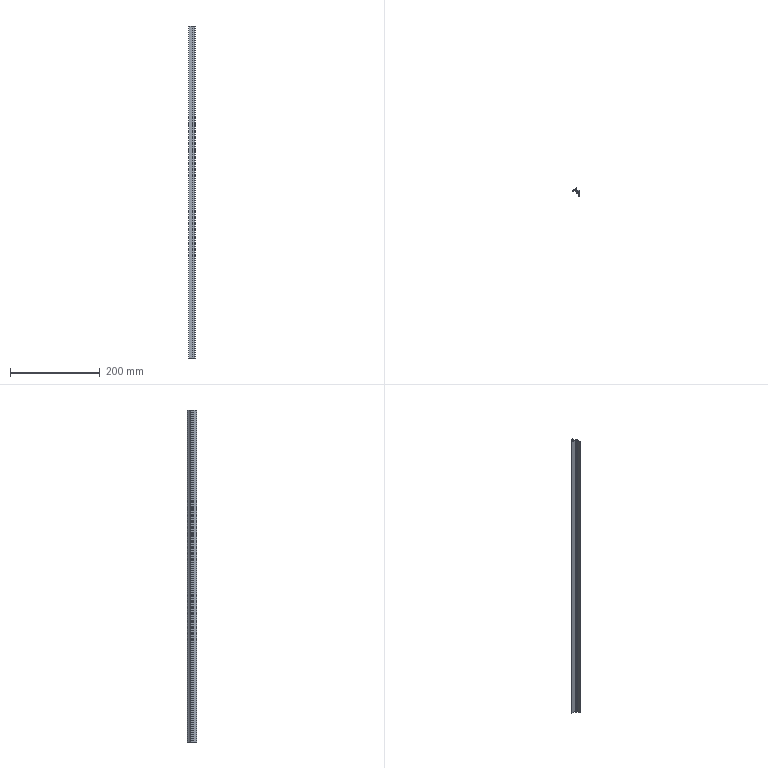Part | SolidWorks | features BaseBody 1, ICE 1, MoveFace 1 | 1 solid | 27 faces | box 14 x 20.3 x 740 mm | volume 37678 mm3 | plane 20 | cylinder 7 | commonest cylinder face diameters 0.387 x2 0.8 x2 0.4 x1 20 x1 22 x1
STEP:
#1=CARTESIAN_POINT('',(-5.304,-0.625,200.));
#2=VERTEX_POINT('',#1);
#3=CARTESIAN_POINT('',(-5.449,-0.8125,200.));
#4=VERTEX_POINT('',#3);
#5=CARTESIAN_POINT('',(-5.255,-0.8125,200.));
#6=DIRECTION('',(0.,0.,1.));
#7=DIRECTION('',(-1.,0.,0.));
#8=AXIS2_PLACEMENT_3D('',#5,#6,#7);
#9=CIRCLE('',#8,0.1937);
#10=EDGE_CURVE('',#2,#4,#9,.T.);
#11=ORIENTED_EDGE('',*,*,#10,.T.);
#12=CARTESIAN_POINT('',(-5.449,-0.8125,-540.));
#13=VERTEX_POINT('',#12);
#14=CARTESIAN_POINT('',(-5.449,-0.8125,230.));
#15=DIRECTION('',(0.,0.,-1.));
#16=VECTOR('',#15,1000.);
#17=LINE('',#14,#16);
#18=EDGE_CURVE('',#4,#13,#17,.T.);
#19=ORIENTED_EDGE('',*,*,#18,.T.);
#20=CARTESIAN_POINT('',(-5.304,-0.625,-540.));
#21=VERTEX_POINT('',#20);
#22=CARTESIAN_POINT('',(-5.255,-0.8125,-540.));
#23=DIRECTION('',(0.,0.,-1.));
#24=DIRECTION('',(1.,0.,0.));
#25=AXIS2_PLACEMENT_3D('',#22,#23,#24);
#26=CIRCLE('',#25,0.1937);
#27=EDGE_CURVE('',#13,#21,#26,.T.);
#28=ORIENTED_EDGE('',*,*,#27,.T.);
#29=CARTESIAN_POINT('',(-5.304,-0.625,230.));
#30=DIRECTION('',(0.,0.,-1.));
#31=VECTOR('',#30,1000.);
#32=LINE('',#29,#31);
#33=EDGE_CURVE('',#2,#21,#32,.T.);
#34=ORIENTED_EDGE('',*,*,#33,.F.);
#35=EDGE_LOOP('',(#11,#19,#28,#34));
#36=FACE_OUTER_BOUND('',#35,.T.);
#37=CARTESIAN_POINT('',(-5.255,-0.8125,230.));
#38=DIRECTION('',(0.,0.,-1.));
#39=DIRECTION('',(-1.,0.,0.));
#40=AXIS2_PLACEMENT_3D('',#37,#38,#39);
#41=CYLINDRICAL_SURFACE('',#40,0.1937);
#42=ADVANCED_FACE('',(#36),#41,.F.);
#43=CARTESIAN_POINT('',(5.,-1.,-540.));
#44=VERTEX_POINT('',#43);
#45=CARTESIAN_POINT('',(5.,-14.3,-540.));
#46=VERTEX_POINT('',#45);
#47=CARTESIAN_POINT('',(5.,29.623,-540.));
#48=DIRECTION('',(0.,-1.,0.));
#49=VECTOR('',#48,1000.);
#50=LINE('',#47,#49);
#51=EDGE_CURVE('',#44,#46,#50,.T.);
#52=ORIENTED_EDGE('',*,*,#51,.F.);
#53=CARTESIAN_POINT('',(5.,-1.,200.));
#54=VERTEX_POINT('',#53);
#55=CARTESIAN_POINT('',(5.,-1.,230.));
#56=DIRECTION('',(0.,0.,-1.));
#57=VECTOR('',#56,1000.);
#58=LINE('',#55,#57);
#59=EDGE_CURVE('',#54,#44,#58,.T.);
#60=ORIENTED_EDGE('',*,*,#59,.F.);
#61=CARTESIAN_POINT('',(5.,-14.3,200.));
#62=VERTEX_POINT('',#61);
#63=CARTESIAN_POINT('',(5.,-14.3,200.));
#64=DIRECTION('',(0.,1.,0.));
#65=VECTOR('',#64,1000.);
#66=LINE('',#63,#65);
#67=EDGE_CURVE('',#62,#54,#66,.T.);
#68=ORIENTED_EDGE('',*,*,#67,.F.);
#69=CARTESIAN_POINT('',(5.,-14.3,230.));
#70=DIRECTION('',(0.,0.,1.));
#71=VECTOR('',#70,1000.);
#72=LINE('',#69,#71);
#73=EDGE_CURVE('',#46,#62,#72,.T.);
#74=ORIENTED_EDGE('',*,*,#73,.F.);
#75=EDGE_LOOP('',(#52,#60,#68,#74));
#76=FACE_OUTER_BOUND('',#75,.T.);
#77=CARTESIAN_POINT('',(5.,-14.3,230.));
#78=DIRECTION('',(-1.,0.,0.));
#79=DIRECTION('',(0.,0.,1.));
#80=AXIS2_PLACEMENT_3D('',#77,#78,#79);
#81=PLANE('',#80);
#82=ADVANCED_FACE('',(#76),#81,.F.);
#83=CARTESIAN_POINT('',(-9.,-2.,-540.));
#84=VERTEX_POINT('',#83);
#85=CARTESIAN_POINT('',(-9.,-2.,200.));
#86=VERTEX_POINT('',#85);
#87=CARTESIAN_POINT('',(-9.,-2.,230.));
#88=DIRECTION('',(0.,0.,1.));
#89=VECTOR('',#88,1000.);
#90=LINE('',#87,#89);
#91=EDGE_CURVE('',#84,#86,#90,.T.);
#92=ORIENTED_EDGE('',*,*,#91,.F.);
#93=CARTESIAN_POINT('',(0.9,-2.,-540.));
#94=VERTEX_POINT('',#93);
#95=CARTESIAN_POINT('',(5.,-2.,-540.));
#96=DIRECTION('',(-1.,0.,0.));
#97=VECTOR('',#96,1000.);
#98=LINE('',#95,#97);
#99=EDGE_CURVE('',#94,#84,#98,.T.);
#100=ORIENTED_EDGE('',*,*,#99,.F.);
#101=CARTESIAN_POINT('',(0.9,-2.,200.));
#102=VERTEX_POINT('',#101);
#103=CARTESIAN_POINT('',(0.9,-2.,230.));
#104=DIRECTION('',(0.,0.,-1.));
#105=VECTOR('',#104,1000.);
#106=LINE('',#103,#105);
#107=EDGE_CURVE('',#102,#94,#106,.T.);
#108=ORIENTED_EDGE('',*,*,#107,.F.);
#109=CARTESIAN_POINT('',(5.,-2.,200.));
#110=DIRECTION('',(1.,0.,0.));
#111=VECTOR('',#110,1000.);
#112=LINE('',#109,#111);
#113=EDGE_CURVE('',#86,#102,#112,.T.);
#114=ORIENTED_EDGE('',*,*,#113,.F.);
#115=EDGE_LOOP('',(#92,#100,#108,#114));
#116=FACE_OUTER_BOUND('',#115,.T.);
#117=CARTESIAN_POINT('',(-9.,-2.,230.));
#118=DIRECTION('',(0.,1.,0.));
#119=DIRECTION('',(0.,0.,1.));
#120=AXIS2_PLACEMENT_3D('',#117,#118,#119);
#121=PLANE('',#120);
#122=ADVANCED_FACE('',(#116),#121,.F.);
#123=CARTESIAN_POINT('',(4.,-6.,200.));
#124=VERTEX_POINT('',#123);
#125=CARTESIAN_POINT('',(4.,-3.,200.));
#126=VERTEX_POINT('',#125);
#127=CARTESIAN_POINT('',(4.,29.623,200.));
#128=DIRECTION('',(0.,1.,0.));
#129=VECTOR('',#128,1000.);
#130=LINE('',#127,#129);
#131=EDGE_CURVE('',#124,#126,#130,.T.);
#132=ORIENTED_EDGE('',*,*,#131,.F.);
#133=CARTESIAN_POINT('',(1.,-6.,200.));
#134=VERTEX_POINT('',#133);
#135=CARTESIAN_POINT('',(5.,-6.,200.));
#136=DIRECTION('',(1.,0.,0.));
#137=VECTOR('',#136,1000.);
#138=LINE('',#135,#137);
#139=EDGE_CURVE('',#134,#124,#138,.T.);
#140=ORIENTED_EDGE('',*,*,#139,.F.);
#141=CARTESIAN_POINT('',(1.,-6.7,200.));
#142=VERTEX_POINT('',#141);
#143=CARTESIAN_POINT('',(1.,-6.,200.));
#144=DIRECTION('',(0.,-1.,0.));
#145=VECTOR('',#144,1000.);
#146=LINE('',#143,#145);
#147=EDGE_CURVE('',#134,#142,#146,.T.);
#148=ORIENTED_EDGE('',*,*,#147,.T.);
#149=CARTESIAN_POINT('',(-1.7,-6.7,200.));
#150=VERTEX_POINT('',#149);
#151=CARTESIAN_POINT('',(5.,-6.7,200.));
#152=DIRECTION('',(1.,0.,0.));
#153=VECTOR('',#152,1000.);
#154=LINE('',#151,#153);
#155=EDGE_CURVE('',#150,#142,#154,.T.);
#156=ORIENTED_EDGE('',*,*,#155,.F.);
#157=CARTESIAN_POINT('',(-1.7,-7.7,200.));
#158=VERTEX_POINT('',#157);
#159=CARTESIAN_POINT('',(-1.7,-6.7,200.));
#160=DIRECTION('',(0.,-1.,0.));
#161=VECTOR('',#160,1000.);
#162=LINE('',#159,#161);
#163=EDGE_CURVE('',#150,#158,#162,.T.);
#164=ORIENTED_EDGE('',*,*,#163,.T.);
#165=CARTESIAN_POINT('',(4.,-7.7,200.));
#166=VERTEX_POINT('',#165);
#167=CARTESIAN_POINT('',(5.,-7.7,200.));
#168=DIRECTION('',(-1.,0.,0.));
#169=VECTOR('',#168,1000.);
#170=LINE('',#167,#169);
#171=EDGE_CURVE('',#166,#158,#170,.T.);
#172=ORIENTED_EDGE('',*,*,#171,.F.);
#173=CARTESIAN_POINT('',(4.,-14.3,200.));
#174=VERTEX_POINT('',#173);
#175=CARTESIAN_POINT('',(4.,29.623,200.));
#176=DIRECTION('',(0.,1.,0.));
#177=VECTOR('',#176,1000.);
#178=LINE('',#175,#177);
#179=EDGE_CURVE('',#174,#166,#178,.T.);
#180=ORIENTED_EDGE('',*,*,#179,.F.);
#181=CARTESIAN_POINT('',(5.,-14.3,200.));
#182=DIRECTION('',(-1.,0.,0.));
#183=VECTOR('',#182,1000.);
#184=LINE('',#181,#183);
#185=EDGE_CURVE('',#62,#174,#184,.T.);
#186=ORIENTED_EDGE('',*,*,#185,.F.);
#187=ORIENTED_EDGE('',*,*,#67,.T.);
#188=CARTESIAN_POINT('',(-5.207,-1.,200.));
#189=VERTEX_POINT('',#188);
#190=CARTESIAN_POINT('',(5.,-1.,200.));
#191=DIRECTION('',(1.,0.,0.));
#192=VECTOR('',#191,1000.);
#193=LINE('',#190,#192);
#194=EDGE_CURVE('',#189,#54,#193,.T.);
#195=ORIENTED_EDGE('',*,*,#194,.F.);
#196=CARTESIAN_POINT('',(-5.255,-0.8125,200.));
#197=DIRECTION('',(0.,0.,1.));
#198=DIRECTION('',(-1.,0.,0.));
#199=AXIS2_PLACEMENT_3D('',#196,#197,#198);
#200=CIRCLE('',#199,0.1937);
#201=EDGE_CURVE('',#4,#189,#200,.T.);
#202=ORIENTED_EDGE('',*,*,#201,.F.);
#203=ORIENTED_EDGE('',*,*,#10,.F.);
#204=CARTESIAN_POINT('',(-1.368,3.063,200.));
#205=VERTEX_POINT('',#204);
#206=CARTESIAN_POINT('',(-10.628,9.,200.));
#207=DIRECTION('',(0.,0.,1.));
#208=DIRECTION('',(-1.,0.,0.));
#209=AXIS2_PLACEMENT_3D('',#206,#207,#208);
#210=CIRCLE('',#209,11.);
#211=EDGE_CURVE('',#2,#205,#210,.T.);
#212=ORIENTED_EDGE('',*,*,#211,.T.);
#213=CARTESIAN_POINT('',(-1.,2.955,200.));
#214=VERTEX_POINT('',#213);
#215=CARTESIAN_POINT('',(-1.2,2.955,200.));
#216=DIRECTION('',(0.,0.,1.));
#217=DIRECTION('',(-1.,0.,0.));
#218=AXIS2_PLACEMENT_3D('',#215,#216,#217);
#219=CIRCLE('',#218,0.2);
#220=EDGE_CURVE('',#214,#205,#219,.T.);
#221=ORIENTED_EDGE('',*,*,#220,.F.);
#222=CARTESIAN_POINT('',(-1.,1.5,200.));
#223=VERTEX_POINT('',#222);
#224=CARTESIAN_POINT('',(-1.,2.955,200.));
#225=DIRECTION('',(0.,1.,0.));
#226=VECTOR('',#225,1000.);
#227=LINE('',#224,#226);
#228=EDGE_CURVE('',#223,#214,#227,.T.);
#229=ORIENTED_EDGE('',*,*,#228,.F.);
#230=CARTESIAN_POINT('',(0.,1.5,200.));
#231=VERTEX_POINT('',#230);
#232=CARTESIAN_POINT('',(-1.,1.5,200.));
#233=DIRECTION('',(-1.,0.,0.));
#234=VECTOR('',#233,1000.);
#235=LINE('',#232,#234);
#236=EDGE_CURVE('',#231,#223,#235,.T.);
#237=ORIENTED_EDGE('',*,*,#236,.F.);
#238=CARTESIAN_POINT('',(0.,6.,200.));
#239=VERTEX_POINT('',#238);
#240=CARTESIAN_POINT('',(0.,1.5,200.));
#241=DIRECTION('',(0.,-1.,0.));
#242=VECTOR('',#241,1000.);
#243=LINE('',#240,#242);
#244=EDGE_CURVE('',#239,#231,#243,.T.);
#245=ORIENTED_EDGE('',*,*,#244,.F.);
#246=CARTESIAN_POINT('',(-0.8,6.,200.));
#247=VERTEX_POINT('',#246);
#248=CARTESIAN_POINT('',(0.,6.,200.));
#249=DIRECTION('',(1.,0.,0.));
#250=VECTOR('',#249,1000.);
#251=LINE('',#248,#250);
#252=EDGE_CURVE('',#247,#239,#251,.T.);
#253=ORIENTED_EDGE('',*,*,#252,.F.);
#254=CARTESIAN_POINT('',(-1.178,5.731,200.));
#255=VERTEX_POINT('',#254);
#256=CARTESIAN_POINT('',(-0.8,5.6,200.));
#257=DIRECTION('',(0.,0.,1.));
#258=DIRECTION('',(-1.,0.,0.));
#259=AXIS2_PLACEMENT_3D('',#256,#257,#258);
#260=CIRCLE('',#259,0.4);
#261=EDGE_CURVE('',#247,#255,#260,.T.);
#262=ORIENTED_EDGE('',*,*,#261,.T.);
#263=CARTESIAN_POINT('',(-8.678,-0.8077,200.));
#264=VERTEX_POINT('',#263);
#265=CARTESIAN_POINT('',(-10.628,9.,200.));
#266=DIRECTION('',(0.,0.,1.));
#267=DIRECTION('',(-1.,0.,0.));
#268=AXIS2_PLACEMENT_3D('',#265,#266,#267);
#269=CIRCLE('',#268,10.);
#270=EDGE_CURVE('',#264,#255,#269,.T.);
#271=ORIENTED_EDGE('',*,*,#270,.F.);
#272=CARTESIAN_POINT('',(-9.,-1.2,200.));
#273=VERTEX_POINT('',#272);
#274=CARTESIAN_POINT('',(-8.6,-1.2,200.));
#275=DIRECTION('',(0.,0.,1.));
#276=DIRECTION('',(-1.,0.,0.));
#277=AXIS2_PLACEMENT_3D('',#274,#275,#276);
#278=CIRCLE('',#277,0.4);
#279=EDGE_CURVE('',#264,#273,#278,.T.);
#280=ORIENTED_EDGE('',*,*,#279,.T.);
#281=CARTESIAN_POINT('',(-9.,8.,200.));
#282=DIRECTION('',(0.,-1.,0.));
#283=VECTOR('',#282,1000.);
#284=LINE('',#281,#283);
#285=EDGE_CURVE('',#273,#86,#284,.T.);
#286=ORIENTED_EDGE('',*,*,#285,.T.);
#287=ORIENTED_EDGE('',*,*,#113,.T.);
#288=CARTESIAN_POINT('',(0.9,-3.,200.));
#289=VERTEX_POINT('',#288);
#290=CARTESIAN_POINT('',(0.9,29.623,200.));
#291=DIRECTION('',(0.,1.,0.));
#292=VECTOR('',#291,1000.);
#293=LINE('',#290,#292);
#294=EDGE_CURVE('',#289,#102,#293,.T.);
#295=ORIENTED_EDGE('',*,*,#294,.F.);
#296=CARTESIAN_POINT('',(5.,-3.,200.));
#297=DIRECTION('',(-1.,0.,0.));
#298=VECTOR('',#297,1000.);
#299=LINE('',#296,#298);
#300=EDGE_CURVE('',#126,#289,#299,.T.);
#301=ORIENTED_EDGE('',*,*,#300,.F.);
#302=EDGE_LOOP('',(#132,#140,#148,#156,#164,#172,#180,#186,#187,#195,#202,#203,#212,#221,#229,#237,#245,#253,#262,#271,#280,#286,#287,#295,#301));
#303=FACE_OUTER_BOUND('',#302,.T.);
#304=CARTESIAN_POINT('',(5.,29.623,200.));
#305=DIRECTION('',(0.,0.,-1.));
#306=DIRECTION('',(-1.,0.,0.));
#307=AXIS2_PLACEMENT_3D('',#304,#305,#306);
#308=PLANE('',#307);
#309=ADVANCED_FACE('',(#303),#308,.F.);
#310=ORIENTED_EDGE('',*,*,#185,.T.);
#311=CARTESIAN_POINT('',(4.,-14.3,-540.));
#312=VERTEX_POINT('',#311);
#313=CARTESIAN_POINT('',(4.,-14.3,230.));
#314=DIRECTION('',(0.,0.,1.));
#315=VECTOR('',#314,1000.);
#316=LINE('',#313,#315);
#317=EDGE_CURVE('',#312,#174,#316,.T.);
#318=ORIENTED_EDGE('',*,*,#317,.F.);
#319=CARTESIAN_POINT('',(5.,-14.3,-540.));
#320=DIRECTION('',(-1.,0.,0.));
#321=VECTOR('',#320,1000.);
#322=LINE('',#319,#321);
#323=EDGE_CURVE('',#46,#312,#322,.T.);
#324=ORIENTED_EDGE('',*,*,#323,.F.);
#325=ORIENTED_EDGE('',*,*,#73,.T.);
#326=EDGE_LOOP('',(#310,#318,#324,#325));
#327=FACE_OUTER_BOUND('',#326,.T.);
#328=CARTESIAN_POINT('',(4.,-14.3,230.));
#329=DIRECTION('',(0.,1.,0.));
#330=DIRECTION('',(0.,0.,1.));
#331=AXIS2_PLACEMENT_3D('',#328,#329,#330);
#332=PLANE('',#331);
#333=ADVANCED_FACE('',(#327),#332,.F.);
#334=ORIENTED_EDGE('',*,*,#51,.T.);
#335=ORIENTED_EDGE('',*,*,#323,.T.);
#336=CARTESIAN_POINT('',(4.,-7.7,-540.));
#337=VERTEX_POINT('',#336);
#338=CARTESIAN_POINT('',(4.,-7.7,-540.));
#339=DIRECTION('',(0.,-1.,0.));
#340=VECTOR('',#339,1000.);
#341=LINE('',#338,#340);
#342=EDGE_CURVE('',#337,#312,#341,.T.);
#343=ORIENTED_EDGE('',*,*,#342,.F.);
#344=CARTESIAN_POINT('',(-1.7,-7.7,-540.));
#345=VERTEX_POINT('',#344);
#346=CARTESIAN_POINT('',(-1.7,-7.7,-540.));
#347=DIRECTION('',(1.,0.,0.));
#348=VECTOR('',#347,1000.);
#349=LINE('',#346,#348);
#350=EDGE_CURVE('',#345,#337,#349,.T.);
#351=ORIENTED_EDGE('',*,*,#350,.F.);
#352=CARTESIAN_POINT('',(-1.7,-6.7,-540.));
#353=VERTEX_POINT('',#352);
#354=CARTESIAN_POINT('',(-1.7,29.623,-540.));
#355=DIRECTION('',(0.,1.,0.));
#356=VECTOR('',#355,1000.);
#357=LINE('',#354,#356);
#358=EDGE_CURVE('',#345,#353,#357,.T.);
#359=ORIENTED_EDGE('',*,*,#358,.T.);
#360=CARTESIAN_POINT('',(1.,-6.7,-540.));
#361=VERTEX_POINT('',#360);
#362=CARTESIAN_POINT('',(1.,-6.7,-540.));
#363=DIRECTION('',(-1.,0.,0.));
#364=VECTOR('',#363,1000.);
#365=LINE('',#362,#364);
#366=EDGE_CURVE('',#361,#353,#365,.T.);
#367=ORIENTED_EDGE('',*,*,#366,.F.);
#368=CARTESIAN_POINT('',(1.,-6.,-540.));
#369=VERTEX_POINT('',#368);
#370=CARTESIAN_POINT('',(1.,29.623,-540.));
#371=DIRECTION('',(0.,1.,0.));
#372=VECTOR('',#371,1000.);
#373=LINE('',#370,#372);
#374=EDGE_CURVE('',#361,#369,#373,.T.);
#375=ORIENTED_EDGE('',*,*,#374,.T.);
#376=CARTESIAN_POINT('',(4.,-6.,-540.));
#377=VERTEX_POINT('',#376);
#378=CARTESIAN_POINT('',(4.,-6.,-540.));
#379=DIRECTION('',(-1.,0.,0.));
#380=VECTOR('',#379,1000.);
#381=LINE('',#378,#380);
#382=EDGE_CURVE('',#377,#369,#381,.T.);
#383=ORIENTED_EDGE('',*,*,#382,.F.);
#384=CARTESIAN_POINT('',(4.,-3.,-540.));
#385=VERTEX_POINT('',#384);
#386=CARTESIAN_POINT('',(4.,-3.,-540.));
#387=DIRECTION('',(0.,-1.,0.));
#388=VECTOR('',#387,1000.);
#389=LINE('',#386,#388);
#390=EDGE_CURVE('',#385,#377,#389,.T.);
#391=ORIENTED_EDGE('',*,*,#390,.F.);
#392=CARTESIAN_POINT('',(0.9,-3.,-540.));
#393=VERTEX_POINT('',#392);
#394=CARTESIAN_POINT('',(0.9,-3.,-540.));
#395=DIRECTION('',(1.,0.,0.));
#396=VECTOR('',#395,1000.);
#397=LINE('',#394,#396);
#398=EDGE_CURVE('',#393,#385,#397,.T.);
#399=ORIENTED_EDGE('',*,*,#398,.F.);
#400=CARTESIAN_POINT('',(0.9,-2.,-540.));
#401=DIRECTION('',(0.,-1.,0.));
#402=VECTOR('',#401,1000.);
#403=LINE('',#400,#402);
#404=EDGE_CURVE('',#94,#393,#403,.T.);
#405=ORIENTED_EDGE('',*,*,#404,.F.);
#406=ORIENTED_EDGE('',*,*,#99,.T.);
#407=CARTESIAN_POINT('',(-9.,-1.2,-540.));
#408=VERTEX_POINT('',#407);
#409=CARTESIAN_POINT('',(-9.,-1.2,-540.));
#410=DIRECTION('',(0.,-1.,0.));
#411=VECTOR('',#410,1000.);
#412=LINE('',#409,#411);
#413=EDGE_CURVE('',#408,#84,#412,.T.);
#414=ORIENTED_EDGE('',*,*,#413,.F.);
#415=CARTESIAN_POINT('',(-8.678,-0.8077,-540.));
#416=VERTEX_POINT('',#415);
#417=CARTESIAN_POINT('',(-8.6,-1.2,-540.));
#418=DIRECTION('',(0.,0.,-1.));
#419=DIRECTION('',(1.,0.,0.));
#420=AXIS2_PLACEMENT_3D('',#417,#418,#419);
#421=CIRCLE('',#420,0.4);
#422=EDGE_CURVE('',#408,#416,#421,.T.);
#423=ORIENTED_EDGE('',*,*,#422,.T.);
#424=CARTESIAN_POINT('',(-1.178,5.731,-540.));
#425=VERTEX_POINT('',#424);
#426=CARTESIAN_POINT('',(-10.628,9.,-540.));
#427=DIRECTION('',(0.,0.,-1.));
#428=DIRECTION('',(1.,0.,0.));
#429=AXIS2_PLACEMENT_3D('',#426,#427,#428);
#430=CIRCLE('',#429,10.);
#431=EDGE_CURVE('',#425,#416,#430,.T.);
#432=ORIENTED_EDGE('',*,*,#431,.F.);
#433=CARTESIAN_POINT('',(-0.8,6.,-540.));
#434=VERTEX_POINT('',#433);
#435=CARTESIAN_POINT('',(-0.8,5.6,-540.));
#436=DIRECTION('',(0.,0.,-1.));
#437=DIRECTION('',(1.,0.,0.));
#438=AXIS2_PLACEMENT_3D('',#435,#436,#437);
#439=CIRCLE('',#438,0.4);
#440=EDGE_CURVE('',#425,#434,#439,.T.);
#441=ORIENTED_EDGE('',*,*,#440,.T.);
#442=CARTESIAN_POINT('',(0.,6.,-540.));
#443=VERTEX_POINT('',#442);
#444=CARTESIAN_POINT('',(0.,6.,-540.));
#445=DIRECTION('',(-1.,0.,0.));
#446=VECTOR('',#445,1000.);
#447=LINE('',#444,#446);
#448=EDGE_CURVE('',#443,#434,#447,.T.);
#449=ORIENTED_EDGE('',*,*,#448,.F.);
#450=CARTESIAN_POINT('',(0.,1.5,-540.));
#451=VERTEX_POINT('',#450);
#452=CARTESIAN_POINT('',(0.,1.5,-540.));
#453=DIRECTION('',(0.,1.,0.));
#454=VECTOR('',#453,1000.);
#455=LINE('',#452,#454);
#456=EDGE_CURVE('',#451,#443,#455,.T.);
#457=ORIENTED_EDGE('',*,*,#456,.F.);
#458=CARTESIAN_POINT('',(-1.,1.5,-540.));
#459=VERTEX_POINT('',#458);
#460=CARTESIAN_POINT('',(-1.,1.5,-540.));
#461=DIRECTION('',(1.,0.,0.));
#462=VECTOR('',#461,1000.);
#463=LINE('',#460,#462);
#464=EDGE_CURVE('',#459,#451,#463,.T.);
#465=ORIENTED_EDGE('',*,*,#464,.F.);
#466=CARTESIAN_POINT('',(-1.,2.955,-540.));
#467=VERTEX_POINT('',#466);
#468=CARTESIAN_POINT('',(-1.,2.955,-540.));
#469=DIRECTION('',(0.,-1.,0.));
#470=VECTOR('',#469,1000.);
#471=LINE('',#468,#470);
#472=EDGE_CURVE('',#467,#459,#471,.T.);
#473=ORIENTED_EDGE('',*,*,#472,.F.);
#474=CARTESIAN_POINT('',(-1.368,3.063,-540.));
#475=VERTEX_POINT('',#474);
#476=CARTESIAN_POINT('',(-1.2,2.955,-540.));
#477=DIRECTION('',(0.,0.,-1.));
#478=DIRECTION('',(1.,0.,0.));
#479=AXIS2_PLACEMENT_3D('',#476,#477,#478);
#480=CIRCLE('',#479,0.2);
#481=EDGE_CURVE('',#475,#467,#480,.T.);
#482=ORIENTED_EDGE('',*,*,#481,.F.);
#483=CARTESIAN_POINT('',(-10.628,9.,-540.));
#484=DIRECTION('',(0.,0.,-1.));
#485=DIRECTION('',(1.,0.,0.));
#486=AXIS2_PLACEMENT_3D('',#483,#484,#485);
#487=CIRCLE('',#486,11.);
#488=EDGE_CURVE('',#475,#21,#487,.T.);
#489=ORIENTED_EDGE('',*,*,#488,.T.);
#490=ORIENTED_EDGE('',*,*,#27,.F.);
#491=CARTESIAN_POINT('',(-5.207,-1.,-540.));
#492=VERTEX_POINT('',#491);
#493=CARTESIAN_POINT('',(-5.255,-0.8125,-540.));
#494=DIRECTION('',(0.,0.,-1.));
#495=DIRECTION('',(1.,0.,0.));
#496=AXIS2_PLACEMENT_3D('',#493,#494,#495);
#497=CIRCLE('',#496,0.1937);
#498=EDGE_CURVE('',#492,#13,#497,.T.);
#499=ORIENTED_EDGE('',*,*,#498,.F.);
#500=CARTESIAN_POINT('',(5.,-1.,-540.));
#501=DIRECTION('',(-1.,0.,0.));
#502=VECTOR('',#501,1000.);
#503=LINE('',#500,#502);
#504=EDGE_CURVE('',#44,#492,#503,.T.);
#505=ORIENTED_EDGE('',*,*,#504,.F.);
#506=EDGE_LOOP('',(#334,#335,#343,#351,#359,#367,#375,#383,#391,#399,#405,#406,#414,#423,#432,#441,#449,#457,#465,#473,#482,#489,#490,#499,#505));
#507=FACE_OUTER_BOUND('',#506,.T.);
#508=CARTESIAN_POINT('',(5.,29.623,-540.));
#509=DIRECTION('',(0.,0.,1.));
#510=DIRECTION('',(1.,0.,0.));
#511=AXIS2_PLACEMENT_3D('',#508,#509,#510);
#512=PLANE('',#511);
#513=ADVANCED_FACE('',(#507),#512,.F.);
#514=ORIENTED_EDGE('',*,*,#59,.T.);
#515=ORIENTED_EDGE('',*,*,#504,.T.);
#516=CARTESIAN_POINT('',(-5.207,-1.,230.));
#517=DIRECTION('',(0.,0.,-1.));
#518=VECTOR('',#517,1000.);
#519=LINE('',#516,#518);
#520=EDGE_CURVE('',#189,#492,#519,.T.);
#521=ORIENTED_EDGE('',*,*,#520,.F.);
#522=ORIENTED_EDGE('',*,*,#194,.T.);
#523=EDGE_LOOP('',(#514,#515,#521,#522));
#524=FACE_OUTER_BOUND('',#523,.T.);
#525=CARTESIAN_POINT('',(5.,-1.,230.));
#526=DIRECTION('',(0.,-1.,0.));
#527=DIRECTION('',(0.,0.,-1.));
#528=AXIS2_PLACEMENT_3D('',#525,#526,#527);
#529=PLANE('',#528);
#530=ADVANCED_FACE('',(#524),#529,.F.);
#531=CARTESIAN_POINT('',(-9.,-1.2,230.));
#532=DIRECTION('',(0.,0.,1.));
#533=VECTOR('',#532,1000.);
#534=LINE('',#531,#533);
#535=EDGE_CURVE('',#408,#273,#534,.T.);
#536=ORIENTED_EDGE('',*,*,#535,.F.);
#537=ORIENTED_EDGE('',*,*,#413,.T.);
#538=ORIENTED_EDGE('',*,*,#91,.T.);
#539=ORIENTED_EDGE('',*,*,#285,.F.);
#540=EDGE_LOOP('',(#536,#537,#538,#539));
#541=FACE_OUTER_BOUND('',#540,.T.);
#542=CARTESIAN_POINT('',(-9.,-1.2,230.));
#543=DIRECTION('',(1.,0.,0.));
#544=DIRECTION('',(0.,0.,-1.));
#545=AXIS2_PLACEMENT_3D('',#542,#543,#544);
#546=PLANE('',#545);
#547=ADVANCED_FACE('',(#541),#546,.F.);
#548=ORIENTED_EDGE('',*,*,#294,.T.);
#549=ORIENTED_EDGE('',*,*,#107,.T.);
#550=ORIENTED_EDGE('',*,*,#404,.T.);
#551=CARTESIAN_POINT('',(0.9,-3.,230.));
#552=DIRECTION('',(0.,0.,-1.));
#553=VECTOR('',#552,1000.);
#554=LINE('',#551,#553);
#555=EDGE_CURVE('',#289,#393,#554,.T.);
#556=ORIENTED_EDGE('',*,*,#555,.F.);
#557=EDGE_LOOP('',(#548,#549,#550,#556));
#558=FACE_OUTER_BOUND('',#557,.T.);
#559=CARTESIAN_POINT('',(0.9,-2.,230.));
#560=DIRECTION('',(1.,0.,0.));
#561=DIRECTION('',(0.,0.,-1.));
#562=AXIS2_PLACEMENT_3D('',#559,#560,#561);
#563=PLANE('',#562);
#564=ADVANCED_FACE('',(#558),#563,.F.);
#565=ORIENTED_EDGE('',*,*,#300,.T.);
#566=ORIENTED_EDGE('',*,*,#555,.T.);
#567=ORIENTED_EDGE('',*,*,#398,.T.);
#568=CARTESIAN_POINT('',(4.,-3.,230.));
#569=DIRECTION('',(0.,0.,-1.));
#570=VECTOR('',#569,1000.);
#571=LINE('',#568,#570);
#572=EDGE_CURVE('',#126,#385,#571,.T.);
#573=ORIENTED_EDGE('',*,*,#572,.F.);
#574=EDGE_LOOP('',(#565,#566,#567,#573));
#575=FACE_OUTER_BOUND('',#574,.T.);
#576=CARTESIAN_POINT('',(0.9,-3.,230.));
#577=DIRECTION('',(0.,1.,0.));
#578=DIRECTION('',(0.,0.,1.));
#579=AXIS2_PLACEMENT_3D('',#576,#577,#578);
#580=PLANE('',#579);
#581=ADVANCED_FACE('',(#575),#580,.F.);
#582=ORIENTED_EDGE('',*,*,#131,.T.);
#583=ORIENTED_EDGE('',*,*,#572,.T.);
#584=ORIENTED_EDGE('',*,*,#390,.T.);
#585=CARTESIAN_POINT('',(4.,-6.,230.));
#586=DIRECTION('',(0.,0.,-1.));
#587=VECTOR('',#586,1000.);
#588=LINE('',#585,#587);
#589=EDGE_CURVE('',#124,#377,#588,.T.);
#590=ORIENTED_EDGE('',*,*,#589,.F.);
#591=EDGE_LOOP('',(#582,#583,#584,#590));
#592=FACE_OUTER_BOUND('',#591,.T.);
#593=CARTESIAN_POINT('',(4.,-3.,230.));
#594=DIRECTION('',(1.,0.,0.));
#595=DIRECTION('',(0.,0.,-1.));
#596=AXIS2_PLACEMENT_3D('',#593,#594,#595);
#597=PLANE('',#596);
#598=ADVANCED_FACE('',(#592),#597,.F.);
#599=ORIENTED_EDGE('',*,*,#139,.T.);
#600=ORIENTED_EDGE('',*,*,#589,.T.);
#601=ORIENTED_EDGE('',*,*,#382,.T.);
#602=CARTESIAN_POINT('',(1.,-6.,230.));
#603=DIRECTION('',(0.,0.,-1.));
#604=VECTOR('',#603,1000.);
#605=LINE('',#602,#604);
#606=EDGE_CURVE('',#134,#369,#605,.T.);
#607=ORIENTED_EDGE('',*,*,#606,.F.);
#608=EDGE_LOOP('',(#599,#600,#601,#607));
#609=FACE_OUTER_BOUND('',#608,.T.);
#610=CARTESIAN_POINT('',(4.,-6.,230.));
#611=DIRECTION('',(0.,-1.,0.));
#612=DIRECTION('',(0.,0.,-1.));
#613=AXIS2_PLACEMENT_3D('',#610,#611,#612);
#614=PLANE('',#613);
#615=ADVANCED_FACE('',(#609),#614,.F.);
#616=ORIENTED_EDGE('',*,*,#155,.T.);
#617=CARTESIAN_POINT('',(1.,-6.7,230.));
#618=DIRECTION('',(0.,0.,1.));
#619=VECTOR('',#618,1000.);
#620=LINE('',#617,#619);
#621=EDGE_CURVE('',#361,#142,#620,.T.);
#622=ORIENTED_EDGE('',*,*,#621,.F.);
#623=ORIENTED_EDGE('',*,*,#366,.T.);
#624=CARTESIAN_POINT('',(-1.7,-6.7,230.));
#625=DIRECTION('',(0.,0.,-1.));
#626=VECTOR('',#625,1000.);
#627=LINE('',#624,#626);
#628=EDGE_CURVE('',#150,#353,#627,.T.);
#629=ORIENTED_EDGE('',*,*,#628,.F.);
#630=EDGE_LOOP('',(#616,#622,#623,#629));
#631=FACE_OUTER_BOUND('',#630,.T.);
#632=CARTESIAN_POINT('',(1.,-6.7,230.));
#633=DIRECTION('',(0.,-1.,0.));
#634=DIRECTION('',(0.,0.,-1.));
#635=AXIS2_PLACEMENT_3D('',#632,#633,#634);
#636=PLANE('',#635);
#637=ADVANCED_FACE('',(#631),#636,.F.);
#638=ORIENTED_EDGE('',*,*,#171,.T.);
#639=CARTESIAN_POINT('',(-1.7,-7.7,230.));
#640=DIRECTION('',(0.,0.,1.));
#641=VECTOR('',#640,1000.);
#642=LINE('',#639,#641);
#643=EDGE_CURVE('',#345,#158,#642,.T.);
#644=ORIENTED_EDGE('',*,*,#643,.F.);
#645=ORIENTED_EDGE('',*,*,#350,.T.);
#646=CARTESIAN_POINT('',(4.,-7.7,230.));
#647=DIRECTION('',(0.,0.,-1.));
#648=VECTOR('',#647,1000.);
#649=LINE('',#646,#648);
#650=EDGE_CURVE('',#166,#337,#649,.T.);
#651=ORIENTED_EDGE('',*,*,#650,.F.);
#652=EDGE_LOOP('',(#638,#644,#645,#651));
#653=FACE_OUTER_BOUND('',#652,.T.);
#654=CARTESIAN_POINT('',(-1.7,-7.7,230.));
#655=DIRECTION('',(0.,1.,0.));
#656=DIRECTION('',(0.,0.,1.));
#657=AXIS2_PLACEMENT_3D('',#654,#655,#656);
#658=PLANE('',#657);
#659=ADVANCED_FACE('',(#653),#658,.F.);
#660=ORIENTED_EDGE('',*,*,#179,.T.);
#661=ORIENTED_EDGE('',*,*,#650,.T.);
#662=ORIENTED_EDGE('',*,*,#342,.T.);
#663=ORIENTED_EDGE('',*,*,#317,.T.);
#664=EDGE_LOOP('',(#660,#661,#662,#663));
#665=FACE_OUTER_BOUND('',#664,.T.);
#666=CARTESIAN_POINT('',(4.,-7.7,230.));
#667=DIRECTION('',(1.,0.,0.));
#668=DIRECTION('',(0.,0.,-1.));
#669=AXIS2_PLACEMENT_3D('',#666,#667,#668);
#670=PLANE('',#669);
#671=ADVANCED_FACE('',(#665),#670,.F.);
#672=ORIENTED_EDGE('',*,*,#18,.F.);
#673=ORIENTED_EDGE('',*,*,#201,.T.);
#674=ORIENTED_EDGE('',*,*,#520,.T.);
#675=ORIENTED_EDGE('',*,*,#498,.T.);
#676=EDGE_LOOP('',(#672,#673,#674,#675));
#677=FACE_OUTER_BOUND('',#676,.T.);
#678=CARTESIAN_POINT('',(-5.255,-0.8125,230.));
#679=DIRECTION('',(0.,0.,-1.));
#680=DIRECTION('',(-1.,0.,0.));
#681=AXIS2_PLACEMENT_3D('',#678,#679,#680);
#682=CYLINDRICAL_SURFACE('',#681,0.1937);
#683=ADVANCED_FACE('',(#677),#682,.F.);
#684=CARTESIAN_POINT('',(-1.,2.955,230.));
#685=DIRECTION('',(0.,0.,1.));
#686=VECTOR('',#685,1000.);
#687=LINE('',#684,#686);
#688=EDGE_CURVE('',#467,#214,#687,.T.);
#689=ORIENTED_EDGE('',*,*,#688,.F.);
#690=ORIENTED_EDGE('',*,*,#472,.T.);
#691=CARTESIAN_POINT('',(-1.,1.5,230.));
#692=DIRECTION('',(0.,0.,-1.));
#693=VECTOR('',#692,1000.);
#694=LINE('',#691,#693);
#695=EDGE_CURVE('',#223,#459,#694,.T.);
#696=ORIENTED_EDGE('',*,*,#695,.F.);
#697=ORIENTED_EDGE('',*,*,#228,.T.);
#698=EDGE_LOOP('',(#689,#690,#696,#697));
#699=FACE_OUTER_BOUND('',#698,.T.);
#700=CARTESIAN_POINT('',(-1.,2.955,230.));
#701=DIRECTION('',(1.,0.,0.));
#702=DIRECTION('',(0.,0.,-1.));
#703=AXIS2_PLACEMENT_3D('',#700,#701,#702);
#704=PLANE('',#703);
#705=ADVANCED_FACE('',(#699),#704,.F.);
#706=ORIENTED_EDGE('',*,*,#488,.F.);
#707=CARTESIAN_POINT('',(-1.368,3.063,230.));
#708=DIRECTION('',(0.,0.,1.));
#709=VECTOR('',#708,1000.);
#710=LINE('',#707,#709);
#711=EDGE_CURVE('',#475,#205,#710,.T.);
#712=ORIENTED_EDGE('',*,*,#711,.T.);
#713=ORIENTED_EDGE('',*,*,#211,.F.);
#714=ORIENTED_EDGE('',*,*,#33,.T.);
#715=EDGE_LOOP('',(#706,#712,#713,#714));
#716=FACE_OUTER_BOUND('',#715,.T.);
#717=CARTESIAN_POINT('',(-10.628,9.,230.));
#718=DIRECTION('',(0.,0.,-1.));
#719=DIRECTION('',(-1.,0.,0.));
#720=AXIS2_PLACEMENT_3D('',#717,#718,#719);
#721=CYLINDRICAL_SURFACE('',#720,11.);
#722=ADVANCED_FACE('',(#716),#721,.T.);
#723=CARTESIAN_POINT('',(-1.178,5.731,230.));
#724=DIRECTION('',(0.,0.,1.));
#725=VECTOR('',#724,1000.);
#726=LINE('',#723,#725);
#727=EDGE_CURVE('',#425,#255,#726,.T.);
#728=ORIENTED_EDGE('',*,*,#727,.F.);
#729=ORIENTED_EDGE('',*,*,#431,.T.);
#730=CARTESIAN_POINT('',(-8.678,-0.8077,230.));
#731=DIRECTION('',(0.,0.,-1.));
#732=VECTOR('',#731,1000.);
#733=LINE('',#730,#732);
#734=EDGE_CURVE('',#264,#416,#733,.T.);
#735=ORIENTED_EDGE('',*,*,#734,.F.);
#736=ORIENTED_EDGE('',*,*,#270,.T.);
#737=EDGE_LOOP('',(#728,#729,#735,#736));
#738=FACE_OUTER_BOUND('',#737,.T.);
#739=CARTESIAN_POINT('',(-10.628,9.,230.));
#740=DIRECTION('',(0.,0.,-1.));
#741=DIRECTION('',(-1.,0.,0.));
#742=AXIS2_PLACEMENT_3D('',#739,#740,#741);
#743=CYLINDRICAL_SURFACE('',#742,10.);
#744=ADVANCED_FACE('',(#738),#743,.F.);
#745=CARTESIAN_POINT('',(0.,1.5,230.));
#746=DIRECTION('',(0.,0.,1.));
#747=VECTOR('',#746,1000.);
#748=LINE('',#745,#747);
#749=EDGE_CURVE('',#451,#231,#748,.T.);
#750=ORIENTED_EDGE('',*,*,#749,.F.);
#751=ORIENTED_EDGE('',*,*,#456,.T.);
#752=CARTESIAN_POINT('',(0.,6.,230.));
#753=DIRECTION('',(0.,0.,-1.));
#754=VECTOR('',#753,1000.);
#755=LINE('',#752,#754);
#756=EDGE_CURVE('',#239,#443,#755,.T.);
#757=ORIENTED_EDGE('',*,*,#756,.F.);
#758=ORIENTED_EDGE('',*,*,#244,.T.);
#759=EDGE_LOOP('',(#750,#751,#757,#758));
#760=FACE_OUTER_BOUND('',#759,.T.);
#761=CARTESIAN_POINT('',(0.,1.5,230.));
#762=DIRECTION('',(-1.,0.,0.));
#763=DIRECTION('',(0.,0.,1.));
#764=AXIS2_PLACEMENT_3D('',#761,#762,#763);
#765=PLANE('',#764);
#766=ADVANCED_FACE('',(#760),#765,.F.);
#767=ORIENTED_EDGE('',*,*,#422,.F.);
#768=ORIENTED_EDGE('',*,*,#535,.T.);
#769=ORIENTED_EDGE('',*,*,#279,.F.);
#770=ORIENTED_EDGE('',*,*,#734,.T.);
#771=EDGE_LOOP('',(#767,#768,#769,#770));
#772=FACE_OUTER_BOUND('',#771,.T.);
#773=CARTESIAN_POINT('',(-8.6,-1.2,230.));
#774=DIRECTION('',(0.,0.,-1.));
#775=DIRECTION('',(-1.,0.,0.));
#776=AXIS2_PLACEMENT_3D('',#773,#774,#775);
#777=CYLINDRICAL_SURFACE('',#776,0.4);
#778=ADVANCED_FACE('',(#772),#777,.T.);
#779=ORIENTED_EDGE('',*,*,#147,.F.);
#780=ORIENTED_EDGE('',*,*,#606,.T.);
#781=ORIENTED_EDGE('',*,*,#374,.F.);
#782=ORIENTED_EDGE('',*,*,#621,.T.);
#783=EDGE_LOOP('',(#779,#780,#781,#782));
#784=FACE_OUTER_BOUND('',#783,.T.);
#785=CARTESIAN_POINT('',(1.,-6.,230.));
#786=DIRECTION('',(1.,0.,0.));
#787=DIRECTION('',(0.,0.,-1.));
#788=AXIS2_PLACEMENT_3D('',#785,#786,#787);
#789=PLANE('',#788);
#790=ADVANCED_FACE('',(#784),#789,.F.);
#791=ORIENTED_EDGE('',*,*,#163,.F.);
#792=ORIENTED_EDGE('',*,*,#628,.T.);
#793=ORIENTED_EDGE('',*,*,#358,.F.);
#794=ORIENTED_EDGE('',*,*,#643,.T.);
#795=EDGE_LOOP('',(#791,#792,#793,#794));
#796=FACE_OUTER_BOUND('',#795,.T.);
#797=CARTESIAN_POINT('',(-1.7,-6.7,230.));
#798=DIRECTION('',(1.,0.,0.));
#799=DIRECTION('',(0.,0.,-1.));
#800=AXIS2_PLACEMENT_3D('',#797,#798,#799);
#801=PLANE('',#800);
#802=ADVANCED_FACE('',(#796),#801,.F.);
#803=ORIENTED_EDGE('',*,*,#711,.F.);
#804=ORIENTED_EDGE('',*,*,#481,.T.);
#805=ORIENTED_EDGE('',*,*,#688,.T.);
#806=ORIENTED_EDGE('',*,*,#220,.T.);
#807=EDGE_LOOP('',(#803,#804,#805,#806));
#808=FACE_OUTER_BOUND('',#807,.T.);
#809=CARTESIAN_POINT('',(-1.2,2.955,230.));
#810=DIRECTION('',(0.,0.,-1.));
#811=DIRECTION('',(-1.,0.,0.));
#812=AXIS2_PLACEMENT_3D('',#809,#810,#811);
#813=CYLINDRICAL_SURFACE('',#812,0.2);
#814=ADVANCED_FACE('',(#808),#813,.F.);
#815=ORIENTED_EDGE('',*,*,#695,.T.);
#816=ORIENTED_EDGE('',*,*,#464,.T.);
#817=ORIENTED_EDGE('',*,*,#749,.T.);
#818=ORIENTED_EDGE('',*,*,#236,.T.);
#819=EDGE_LOOP('',(#815,#816,#817,#818));
#820=FACE_OUTER_BOUND('',#819,.T.);
#821=CARTESIAN_POINT('',(-1.,1.5,230.));
#822=DIRECTION('',(0.,1.,0.));
#823=DIRECTION('',(0.,0.,1.));
#824=AXIS2_PLACEMENT_3D('',#821,#822,#823);
#825=PLANE('',#824);
#826=ADVANCED_FACE('',(#820),#825,.F.);
#827=ORIENTED_EDGE('',*,*,#440,.F.);
#828=ORIENTED_EDGE('',*,*,#727,.T.);
#829=ORIENTED_EDGE('',*,*,#261,.F.);
#830=CARTESIAN_POINT('',(-0.8,6.,230.));
#831=DIRECTION('',(0.,0.,-1.));
#832=VECTOR('',#831,1000.);
#833=LINE('',#830,#832);
#834=EDGE_CURVE('',#247,#434,#833,.T.);
#835=ORIENTED_EDGE('',*,*,#834,.T.);
#836=EDGE_LOOP('',(#827,#828,#829,#835));
#837=FACE_OUTER_BOUND('',#836,.T.);
#838=CARTESIAN_POINT('',(-0.8,5.6,230.));
#839=DIRECTION('',(0.,0.,-1.));
#840=DIRECTION('',(-1.,0.,0.));
#841=AXIS2_PLACEMENT_3D('',#838,#839,#840);
#842=CYLINDRICAL_SURFACE('',#841,0.4);
#843=ADVANCED_FACE('',(#837),#842,.T.);
#844=ORIENTED_EDGE('',*,*,#756,.T.);
#845=ORIENTED_EDGE('',*,*,#448,.T.);
#846=ORIENTED_EDGE('',*,*,#834,.F.);
#847=ORIENTED_EDGE('',*,*,#252,.T.);
#848=EDGE_LOOP('',(#844,#845,#846,#847));
#849=FACE_OUTER_BOUND('',#848,.T.);
#850=CARTESIAN_POINT('',(0.,6.,230.));
#851=DIRECTION('',(0.,-1.,0.));
#852=DIRECTION('',(0.,0.,-1.));
#853=AXIS2_PLACEMENT_3D('',#850,#851,#852);
#854=PLANE('',#853);
#855=ADVANCED_FACE('',(#849),#854,.F.);
#856=CLOSED_SHELL('',(#42,#82,#122,#309,#333,#513,#530,#547,#564,#581,#598,#615,#637,#659,#671,#683,#705,#722,#744,#766,#778,#790,#802,#814,#826,#843,#855));
#857=MANIFOLD_SOLID_BREP('',#856);
#858=CARTESIAN_POINT('',(0.,0.,0.));
#859=DIRECTION('',(0.,0.,1.));
#860=DIRECTION('',(1.,0.,0.));
#861=AXIS2_PLACEMENT_3D('',#858,#859,#860);
#862=(LENGTH_UNIT()NAMED_UNIT(*)SI_UNIT(.MILLI.,.METRE.));
#863=UNCERTAINTY_MEASURE_WITH_UNIT(LENGTH_MEASURE(0.00001),#862,'','');
#864=(NAMED_UNIT(*)PLANE_ANGLE_UNIT()SI_UNIT($,.RADIAN.));
#865=(NAMED_UNIT(*)SI_UNIT($,.STERADIAN.)SOLID_ANGLE_UNIT());
#866=(GEOMETRIC_REPRESENTATION_CONTEXT(3)GLOBAL_UNCERTAINTY_ASSIGNED_CONTEXT((#863))GLOBAL_UNIT_ASSIGNED_CONTEXT((#862,#864,#865))REPRESENTATION_CONTEXT('',''));
#867=ADVANCED_BREP_SHAPE_REPRESENTATION('',(#857,#861),#866);